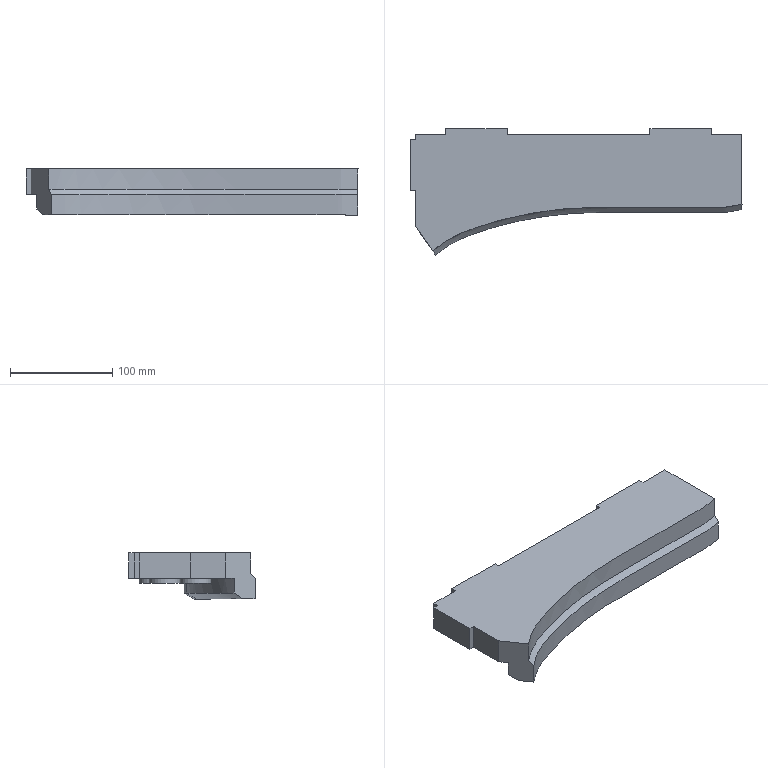Part | NX | features solid 2 | 1 solid | 34 faces | box 324.75 x 123.376 x 45.358 mm | volume 828715 mm3 | plane 23 | spline 6 | cylinder 5 | commonest cylinder face diameters 30 x5